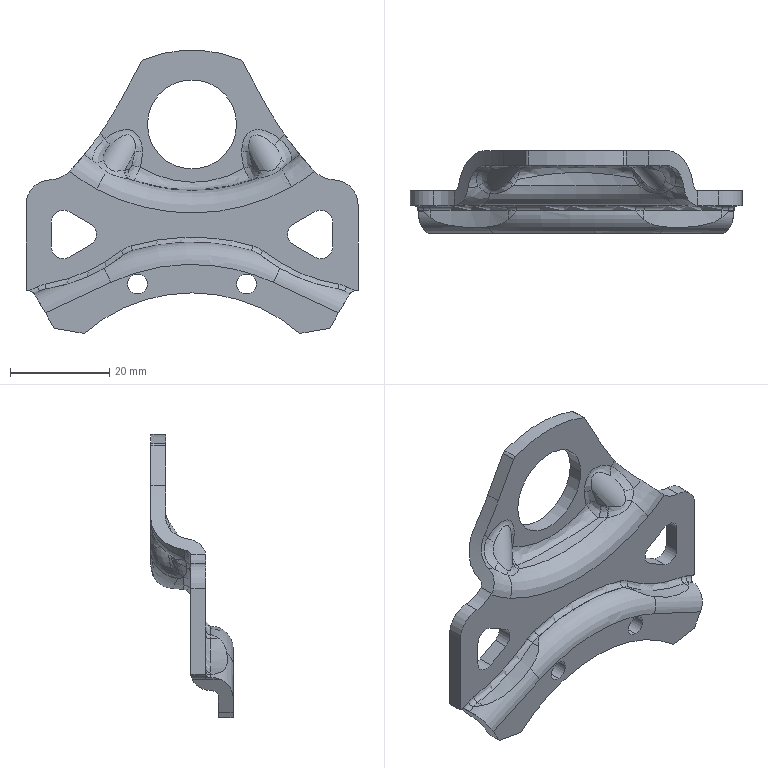Part | NX | features BREP 1 | 1 solid | 214 faces | box 67 x 16.6 x 57.2 mm | volume 7817 mm3 | cylinder 67 | spline 56 | plane 42 | torus 35 | cone 14 | commonest cylinder face diameters 0.6 x12 4 x10 4.8 x6 10 x6 1 x4 2 x4